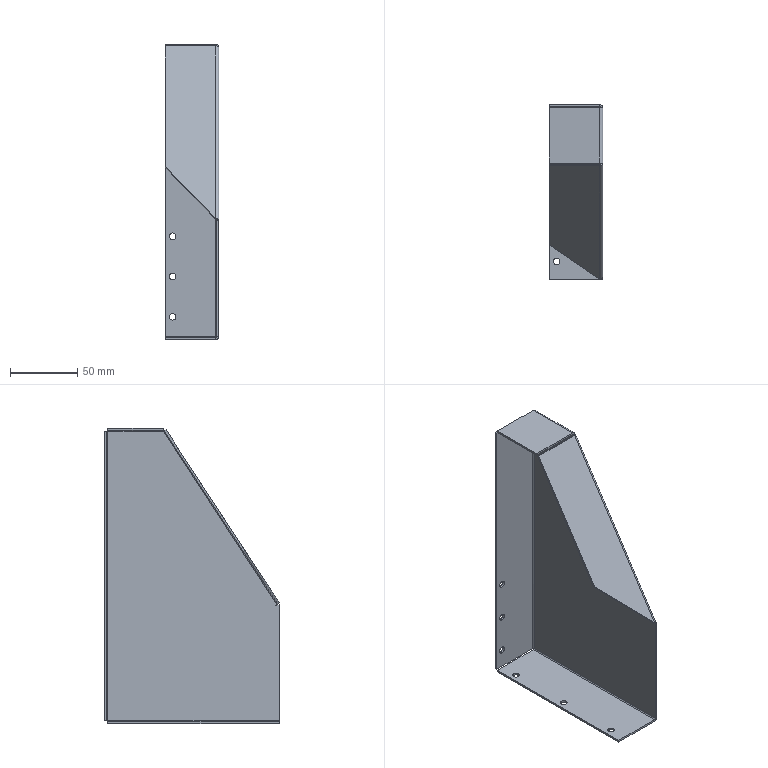Part | STEP file | 1 solid | 54 faces | box 40 x 130 x 220 mm | volume 63688 mm3 | plane 28 | cylinder 20 | spline 6 | commonest cylinder face diameters 5 x12 1.473 x4 4.473 x4